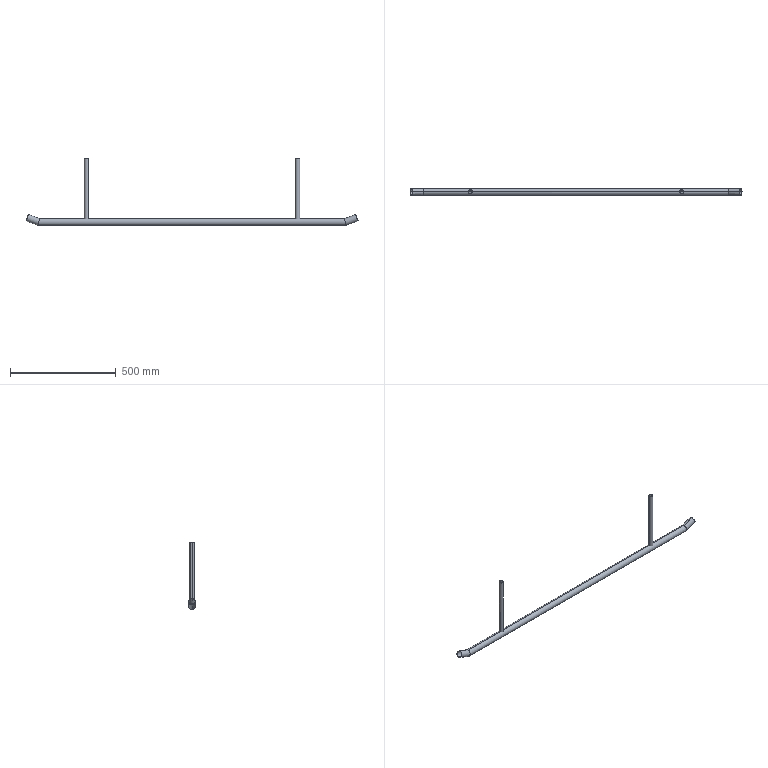Part | STEP file | 14-Guardrail_default<machined> | 5 solids | 30 faces | box 1571 x 32 x 316 mm | volume 277538 mm3 | cylinder 20 | plane 10 | commonest cylinder face diameters 29 x6 32 x6 17 x4 20 x4